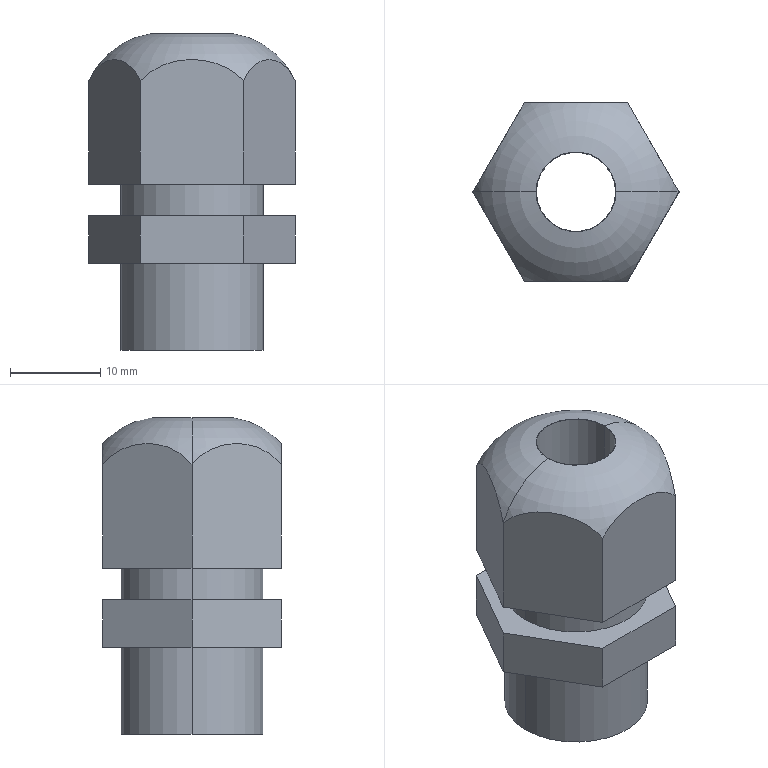Part | SolidWorks | features BaseBody 1 | 1 solid | 29 faces | box 22.88 x 19.815 x 35.2 mm | volume 6256 mm3 | plane 17 | cylinder 8 | cone 2 | torus 2 | commonest cylinder face diameters 15.84 x4 8.8 x2 12.32 x2
STEP:
#1=CARTESIAN_POINT('',(6.16,0.,21.12));
#2=VERTEX_POINT('',#1);
#3=CARTESIAN_POINT('',(-6.16,0.,21.12));
#4=VERTEX_POINT('',#3);
#5=CARTESIAN_POINT('',(0.,0.,21.12));
#6=DIRECTION('',(0.,0.,-1.));
#7=DIRECTION('',(-1.,0.,0.));
#8=AXIS2_PLACEMENT_3D('',#5,#6,#7);
#9=CIRCLE('',#8,6.16);
#10=EDGE_CURVE('',#2,#4,#9,.T.);
#11=ORIENTED_EDGE('',*,*,#10,.F.);
#12=CARTESIAN_POINT('',(6.16,0.,0.));
#13=VERTEX_POINT('',#12);
#14=CARTESIAN_POINT('',(6.16,0.,0.));
#15=DIRECTION('',(0.,0.,-1.));
#16=VECTOR('',#15,1000.);
#17=LINE('',#14,#16);
#18=EDGE_CURVE('',#2,#13,#17,.T.);
#19=ORIENTED_EDGE('',*,*,#18,.T.);
#20=CARTESIAN_POINT('',(-6.16,0.,0.));
#21=VERTEX_POINT('',#20);
#22=CARTESIAN_POINT('',(0.,0.,0.));
#23=DIRECTION('',(0.,0.,1.));
#24=DIRECTION('',(-1.,0.,0.));
#25=AXIS2_PLACEMENT_3D('',#22,#23,#24);
#26=CIRCLE('',#25,6.16);
#27=EDGE_CURVE('',#21,#13,#26,.T.);
#28=ORIENTED_EDGE('',*,*,#27,.F.);
#29=CARTESIAN_POINT('',(-6.16,0.,0.));
#30=DIRECTION('',(0.,0.,-1.));
#31=VECTOR('',#30,1000.);
#32=LINE('',#29,#31);
#33=EDGE_CURVE('',#4,#21,#32,.T.);
#34=ORIENTED_EDGE('',*,*,#33,.F.);
#35=EDGE_LOOP('',(#11,#19,#28,#34));
#36=FACE_OUTER_BOUND('',#35,.T.);
#37=CARTESIAN_POINT('',(0.,0.,0.));
#38=DIRECTION('',(0.,0.,-1.));
#39=DIRECTION('',(-1.,0.,0.));
#40=AXIS2_PLACEMENT_3D('',#37,#38,#39);
#41=CYLINDRICAL_SURFACE('',#40,6.16);
#42=ADVANCED_FACE('',(#36),#41,.F.);
#43=CARTESIAN_POINT('',(4.4,0.,22.754));
#44=VERTEX_POINT('',#43);
#45=CARTESIAN_POINT('',(-4.4,0.,22.754));
#46=VERTEX_POINT('',#45);
#47=CARTESIAN_POINT('',(0.,0.,22.754));
#48=DIRECTION('',(0.,0.,-1.));
#49=DIRECTION('',(1.,0.,0.));
#50=AXIS2_PLACEMENT_3D('',#47,#48,#49);
#51=CIRCLE('',#50,4.4);
#52=EDGE_CURVE('',#44,#46,#51,.T.);
#53=ORIENTED_EDGE('',*,*,#52,.F.);
#54=CARTESIAN_POINT('',(6.16,0.,21.12));
#55=DIRECTION('',(0.7329,0.,-0.6804));
#56=VECTOR('',#55,1000.);
#57=LINE('',#54,#56);
#58=EDGE_CURVE('',#44,#2,#57,.T.);
#59=ORIENTED_EDGE('',*,*,#58,.T.);
#60=ORIENTED_EDGE('',*,*,#10,.T.);
#61=CARTESIAN_POINT('',(-6.16,0.,21.12));
#62=DIRECTION('',(-0.7329,0.,-0.6804));
#63=VECTOR('',#62,1000.);
#64=LINE('',#61,#63);
#65=EDGE_CURVE('',#46,#4,#64,.T.);
#66=ORIENTED_EDGE('',*,*,#65,.F.);
#67=EDGE_LOOP('',(#53,#59,#60,#66));
#68=FACE_OUTER_BOUND('',#67,.T.);
#69=CARTESIAN_POINT('',(0.,0.,21.12));
#70=DIRECTION('',(0.,0.,-1.));
#71=DIRECTION('',(-1.,0.,0.));
#72=AXIS2_PLACEMENT_3D('',#69,#70,#71);
#73=CONICAL_SURFACE('',#72,6.16,0.8225);
#74=ADVANCED_FACE('',(#68),#73,.F.);
#75=CARTESIAN_POINT('',(-7.92,0.,9.68));
#76=VERTEX_POINT('',#75);
#77=CARTESIAN_POINT('',(7.92,0.,9.68));
#78=VERTEX_POINT('',#77);
#79=CARTESIAN_POINT('',(0.,0.,9.68));
#80=DIRECTION('',(0.,0.,-1.));
#81=DIRECTION('',(-1.,0.,0.));
#82=AXIS2_PLACEMENT_3D('',#79,#80,#81);
#83=CIRCLE('',#82,7.92);
#84=EDGE_CURVE('',#76,#78,#83,.T.);
#85=ORIENTED_EDGE('',*,*,#84,.T.);
#86=CARTESIAN_POINT('',(7.92,0.,0.));
#87=VERTEX_POINT('',#86);
#88=CARTESIAN_POINT('',(7.92,0.,0.));
#89=DIRECTION('',(0.,0.,-1.));
#90=VECTOR('',#89,1000.);
#91=LINE('',#88,#90);
#92=EDGE_CURVE('',#78,#87,#91,.T.);
#93=ORIENTED_EDGE('',*,*,#92,.T.);
#94=CARTESIAN_POINT('',(-7.92,0.,0.));
#95=VERTEX_POINT('',#94);
#96=CARTESIAN_POINT('',(0.,0.,0.));
#97=DIRECTION('',(0.,0.,1.));
#98=DIRECTION('',(-1.,0.,0.));
#99=AXIS2_PLACEMENT_3D('',#96,#97,#98);
#100=CIRCLE('',#99,7.92);
#101=EDGE_CURVE('',#87,#95,#100,.T.);
#102=ORIENTED_EDGE('',*,*,#101,.T.);
#103=CARTESIAN_POINT('',(-7.92,0.,0.));
#104=DIRECTION('',(0.,0.,-1.));
#105=VECTOR('',#104,1000.);
#106=LINE('',#103,#105);
#107=EDGE_CURVE('',#76,#95,#106,.T.);
#108=ORIENTED_EDGE('',*,*,#107,.F.);
#109=EDGE_LOOP('',(#85,#93,#102,#108));
#110=FACE_OUTER_BOUND('',#109,.T.);
#111=CARTESIAN_POINT('',(0.,0.,0.));
#112=DIRECTION('',(0.,0.,-1.));
#113=DIRECTION('',(-1.,0.,0.));
#114=AXIS2_PLACEMENT_3D('',#111,#112,#113);
#115=CYLINDRICAL_SURFACE('',#114,7.92);
#116=ADVANCED_FACE('',(#110),#115,.T.);
#117=CARTESIAN_POINT('',(4.4,0.,35.2));
#118=VERTEX_POINT('',#117);
#119=CARTESIAN_POINT('',(-4.4,0.,35.2));
#120=VERTEX_POINT('',#119);
#121=CARTESIAN_POINT('',(0.,0.,35.2));
#122=DIRECTION('',(0.,0.,-1.));
#123=DIRECTION('',(-1.,0.,0.));
#124=AXIS2_PLACEMENT_3D('',#121,#122,#123);
#125=CIRCLE('',#124,4.4);
#126=EDGE_CURVE('',#118,#120,#125,.T.);
#127=ORIENTED_EDGE('',*,*,#126,.F.);
#128=CARTESIAN_POINT('',(4.4,0.,0.));
#129=DIRECTION('',(0.,0.,-1.));
#130=VECTOR('',#129,1000.);
#131=LINE('',#128,#130);
#132=EDGE_CURVE('',#118,#44,#131,.T.);
#133=ORIENTED_EDGE('',*,*,#132,.T.);
#134=ORIENTED_EDGE('',*,*,#52,.T.);
#135=CARTESIAN_POINT('',(-4.4,0.,0.));
#136=DIRECTION('',(0.,0.,-1.));
#137=VECTOR('',#136,1000.);
#138=LINE('',#135,#137);
#139=EDGE_CURVE('',#120,#46,#138,.T.);
#140=ORIENTED_EDGE('',*,*,#139,.F.);
#141=EDGE_LOOP('',(#127,#133,#134,#140));
#142=FACE_OUTER_BOUND('',#141,.T.);
#143=CARTESIAN_POINT('',(0.,0.,0.));
#144=DIRECTION('',(0.,0.,-1.));
#145=DIRECTION('',(-1.,0.,0.));
#146=AXIS2_PLACEMENT_3D('',#143,#144,#145);
#147=CYLINDRICAL_SURFACE('',#146,4.4);
#148=ADVANCED_FACE('',(#142),#147,.F.);
#149=CARTESIAN_POINT('',(-5.72,9.907,29.944));
#150=VERTEX_POINT('',#149);
#151=CARTESIAN_POINT('',(-11.44,0.,29.944));
#152=VERTEX_POINT('',#151);
#153=CARTESIAN_POINT('',(-5.72,9.907,29.944));
#154=CARTESIAN_POINT('',(-5.898,9.599,30.347));
#155=CARTESIAN_POINT('',(-6.098,9.252,30.693));
#156=CARTESIAN_POINT('',(-6.536,8.494,31.288));
#157=CARTESIAN_POINT('',(-6.776,8.078,31.538));
#158=CARTESIAN_POINT('',(-7.27,7.223,31.929));
#159=CARTESIAN_POINT('',(-7.525,6.78,32.073));
#160=CARTESIAN_POINT('',(-8.052,5.868,32.266));
#161=CARTESIAN_POINT('',(-8.317,5.41,32.312));
#162=CARTESIAN_POINT('',(-8.714,4.722,32.312));
#163=CARTESIAN_POINT('',(-8.847,4.492,32.3));
#164=CARTESIAN_POINT('',(-9.113,4.031,32.252));
#165=CARTESIAN_POINT('',(-9.246,3.801,32.215));
#166=CARTESIAN_POINT('',(-9.637,3.123,32.071));
#167=CARTESIAN_POINT('',(-9.891,2.683,31.928));
#168=CARTESIAN_POINT('',(-10.383,1.832,31.539));
#169=CARTESIAN_POINT('',(-10.623,1.415,31.289));
#170=CARTESIAN_POINT('',(-11.061,0.6558,30.693));
#171=CARTESIAN_POINT('',(-11.262,0.3088,30.347));
#172=CARTESIAN_POINT('',(-11.44,0.,29.944));
#173=B_SPLINE_CURVE_WITH_KNOTS('',3,(#153,#154,#155,#156,#157,#158,#159,#160,#161,#162,#163,#164,#165,#166,#167,#168,#169,#170,#171,#172),.UNSPECIFIED.,.F.,.F.,(4,2,2,2,2,2,2,2,2,4),(0.,0.001585,0.00317,0.004755,0.00634,0.007132,0.007924,0.009509,0.01109,0.01268),.UNSPECIFIED.);
#174=EDGE_CURVE('',#150,#152,#173,.T.);
#175=ORIENTED_EDGE('',*,*,#174,.T.);
#176=CARTESIAN_POINT('',(-4.446,0.,35.2));
#177=VERTEX_POINT('',#176);
#178=CARTESIAN_POINT('',(-3.243,0.,26.318));
#179=DIRECTION('',(0.,1.,0.));
#180=DIRECTION('',(-1.,0.,0.));
#181=AXIS2_PLACEMENT_3D('',#178,#179,#180);
#182=CIRCLE('',#181,8.963);
#183=EDGE_CURVE('',#152,#177,#182,.T.);
#184=ORIENTED_EDGE('',*,*,#183,.T.);
#185=CARTESIAN_POINT('',(4.446,0.,35.2));
#186=VERTEX_POINT('',#185);
#187=CARTESIAN_POINT('',(0.,0.,35.2));
#188=DIRECTION('',(0.,0.,1.));
#189=DIRECTION('',(1.,0.,0.));
#190=AXIS2_PLACEMENT_3D('',#187,#188,#189);
#191=CIRCLE('',#190,4.446);
#192=EDGE_CURVE('',#186,#177,#191,.T.);
#193=ORIENTED_EDGE('',*,*,#192,.F.);
#194=CARTESIAN_POINT('',(11.44,0.,29.944));
#195=VERTEX_POINT('',#194);
#196=CARTESIAN_POINT('',(3.243,0.,26.318));
#197=DIRECTION('',(0.,-1.,0.));
#198=DIRECTION('',(0.,0.,-1.));
#199=AXIS2_PLACEMENT_3D('',#196,#197,#198);
#200=CIRCLE('',#199,8.963);
#201=EDGE_CURVE('',#195,#186,#200,.T.);
#202=ORIENTED_EDGE('',*,*,#201,.F.);
#203=CARTESIAN_POINT('',(5.72,9.907,29.944));
#204=VERTEX_POINT('',#203);
#205=CARTESIAN_POINT('',(11.44,0.,29.944));
#206=CARTESIAN_POINT('',(11.262,0.3085,30.347));
#207=CARTESIAN_POINT('',(11.062,0.6552,30.693));
#208=CARTESIAN_POINT('',(10.624,1.413,31.288));
#209=CARTESIAN_POINT('',(10.384,1.829,31.538));
#210=CARTESIAN_POINT('',(9.89,2.684,31.929));
#211=CARTESIAN_POINT('',(9.635,3.127,32.073));
#212=CARTESIAN_POINT('',(9.108,4.04,32.266));
#213=CARTESIAN_POINT('',(8.843,4.497,32.312));
#214=CARTESIAN_POINT('',(8.446,5.186,32.312));
#215=CARTESIAN_POINT('',(8.313,5.416,32.3));
#216=CARTESIAN_POINT('',(8.047,5.876,32.252));
#217=CARTESIAN_POINT('',(7.914,6.106,32.215));
#218=CARTESIAN_POINT('',(7.523,6.784,32.071));
#219=CARTESIAN_POINT('',(7.269,7.224,31.928));
#220=CARTESIAN_POINT('',(6.777,8.076,31.539));
#221=CARTESIAN_POINT('',(6.537,8.492,31.289));
#222=CARTESIAN_POINT('',(6.099,9.252,30.693));
#223=CARTESIAN_POINT('',(5.898,9.599,30.347));
#224=CARTESIAN_POINT('',(5.72,9.907,29.944));
#225=B_SPLINE_CURVE_WITH_KNOTS('',3,(#205,#206,#207,#208,#209,#210,#211,#212,#213,#214,#215,#216,#217,#218,#219,#220,#221,#222,#223,#224),.UNSPECIFIED.,.F.,.F.,(4,2,2,2,2,2,2,2,2,4),(0.,0.001585,0.00317,0.004755,0.00634,0.007132,0.007924,0.009509,0.01109,0.01268),.UNSPECIFIED.);
#226=EDGE_CURVE('',#195,#204,#225,.T.);
#227=ORIENTED_EDGE('',*,*,#226,.T.);
#228=CARTESIAN_POINT('',(5.72,9.907,29.944));
#229=CARTESIAN_POINT('',(5.364,9.907,30.347));
#230=CARTESIAN_POINT('',(4.963,9.907,30.693));
#231=CARTESIAN_POINT('',(4.088,9.907,31.288));
#232=CARTESIAN_POINT('',(3.608,9.907,31.538));
#233=CARTESIAN_POINT('',(2.621,9.907,31.929));
#234=CARTESIAN_POINT('',(2.109,9.907,32.073));
#235=CARTESIAN_POINT('',(1.056,9.907,32.266));
#236=CARTESIAN_POINT('',(0.527,9.907,32.312));
#237=CARTESIAN_POINT('',(-0.2681,9.907,32.312));
#238=CARTESIAN_POINT('',(-0.5335,9.907,32.3));
#239=CARTESIAN_POINT('',(-1.065,9.907,32.252));
#240=CARTESIAN_POINT('',(-1.331,9.907,32.215));
#241=CARTESIAN_POINT('',(-2.114,9.907,32.071));
#242=CARTESIAN_POINT('',(-2.621,9.907,31.928));
#243=CARTESIAN_POINT('',(-3.605,9.907,31.539));
#244=CARTESIAN_POINT('',(-4.086,9.907,31.289));
#245=CARTESIAN_POINT('',(-4.963,9.907,30.693));
#246=CARTESIAN_POINT('',(-5.363,9.907,30.347));
#247=CARTESIAN_POINT('',(-5.72,9.907,29.944));
#248=B_SPLINE_CURVE_WITH_KNOTS('',3,(#228,#229,#230,#231,#232,#233,#234,#235,#236,#237,#238,#239,#240,#241,#242,#243,#244,#245,#246,#247),.UNSPECIFIED.,.F.,.F.,(4,2,2,2,2,2,2,2,2,4),(0.,0.001585,0.00317,0.004755,0.00634,0.007132,0.007924,0.009509,0.01109,0.01268),.UNSPECIFIED.);
#249=EDGE_CURVE('',#204,#150,#248,.T.);
#250=ORIENTED_EDGE('',*,*,#249,.T.);
#251=EDGE_LOOP('',(#175,#184,#193,#202,#227,#250));
#252=FACE_OUTER_BOUND('',#251,.T.);
#253=CARTESIAN_POINT('',(0.,0.,26.318));
#254=DIRECTION('',(0.,0.,1.));
#255=DIRECTION('',(1.,0.,0.));
#256=AXIS2_PLACEMENT_3D('',#253,#254,#255);
#257=TOROIDAL_SURFACE('',#256,3.243,8.963);
#258=ADVANCED_FACE('',(#252),#257,.T.);
#259=CARTESIAN_POINT('',(-7.92,0.,18.48));
#260=VERTEX_POINT('',#259);
#261=CARTESIAN_POINT('',(7.92,0.,18.48));
#262=VERTEX_POINT('',#261);
#263=CARTESIAN_POINT('',(0.,0.,18.48));
#264=DIRECTION('',(0.,0.,-1.));
#265=DIRECTION('',(-1.,0.,0.));
#266=AXIS2_PLACEMENT_3D('',#263,#264,#265);
#267=CIRCLE('',#266,7.92);
#268=EDGE_CURVE('',#260,#262,#267,.T.);
#269=ORIENTED_EDGE('',*,*,#268,.T.);
#270=CARTESIAN_POINT('',(7.92,0.,14.96));
#271=VERTEX_POINT('',#270);
#272=CARTESIAN_POINT('',(7.92,0.,0.));
#273=DIRECTION('',(0.,0.,-1.));
#274=VECTOR('',#273,1000.);
#275=LINE('',#272,#274);
#276=EDGE_CURVE('',#262,#271,#275,.T.);
#277=ORIENTED_EDGE('',*,*,#276,.T.);
#278=CARTESIAN_POINT('',(-7.92,0.,14.96));
#279=VERTEX_POINT('',#278);
#280=CARTESIAN_POINT('',(0.,0.,14.96));
#281=DIRECTION('',(0.,0.,1.));
#282=DIRECTION('',(-1.,0.,0.));
#283=AXIS2_PLACEMENT_3D('',#280,#281,#282);
#284=CIRCLE('',#283,7.92);
#285=EDGE_CURVE('',#271,#279,#284,.T.);
#286=ORIENTED_EDGE('',*,*,#285,.T.);
#287=CARTESIAN_POINT('',(-7.92,0.,0.));
#288=DIRECTION('',(0.,0.,-1.));
#289=VECTOR('',#288,1000.);
#290=LINE('',#287,#289);
#291=EDGE_CURVE('',#260,#279,#290,.T.);
#292=ORIENTED_EDGE('',*,*,#291,.F.);
#293=EDGE_LOOP('',(#269,#277,#286,#292));
#294=FACE_OUTER_BOUND('',#293,.T.);
#295=CARTESIAN_POINT('',(0.,0.,0.));
#296=DIRECTION('',(0.,0.,-1.));
#297=DIRECTION('',(-1.,0.,0.));
#298=AXIS2_PLACEMENT_3D('',#295,#296,#297);
#299=CYLINDRICAL_SURFACE('',#298,7.92);
#300=ADVANCED_FACE('',(#294),#299,.T.);
#301=ORIENTED_EDGE('',*,*,#18,.F.);
#302=CARTESIAN_POINT('',(0.,0.,21.12));
#303=DIRECTION('',(0.,0.,-1.));
#304=DIRECTION('',(-1.,0.,0.));
#305=AXIS2_PLACEMENT_3D('',#302,#303,#304);
#306=CIRCLE('',#305,6.16);
#307=EDGE_CURVE('',#4,#2,#306,.T.);
#308=ORIENTED_EDGE('',*,*,#307,.F.);
#309=ORIENTED_EDGE('',*,*,#33,.T.);
#310=CARTESIAN_POINT('',(0.,0.,0.));
#311=DIRECTION('',(0.,0.,1.));
#312=DIRECTION('',(-1.,0.,0.));
#313=AXIS2_PLACEMENT_3D('',#310,#311,#312);
#314=CIRCLE('',#313,6.16);
#315=EDGE_CURVE('',#13,#21,#314,.T.);
#316=ORIENTED_EDGE('',*,*,#315,.F.);
#317=EDGE_LOOP('',(#301,#308,#309,#316));
#318=FACE_OUTER_BOUND('',#317,.T.);
#319=CARTESIAN_POINT('',(0.,0.,0.));
#320=DIRECTION('',(0.,0.,-1.));
#321=DIRECTION('',(-1.,0.,0.));
#322=AXIS2_PLACEMENT_3D('',#319,#320,#321);
#323=CYLINDRICAL_SURFACE('',#322,6.16);
#324=ADVANCED_FACE('',(#318),#323,.F.);
#325=ORIENTED_EDGE('',*,*,#27,.T.);
#326=ORIENTED_EDGE('',*,*,#315,.T.);
#327=EDGE_LOOP('',(#325,#326));
#328=FACE_BOUND('',#327,.T.);
#329=CARTESIAN_POINT('',(0.,0.,0.));
#330=DIRECTION('',(0.,0.,1.));
#331=DIRECTION('',(-1.,0.,0.));
#332=AXIS2_PLACEMENT_3D('',#329,#330,#331);
#333=CIRCLE('',#332,7.92);
#334=EDGE_CURVE('',#95,#87,#333,.T.);
#335=ORIENTED_EDGE('',*,*,#334,.F.);
#336=ORIENTED_EDGE('',*,*,#101,.F.);
#337=EDGE_LOOP('',(#335,#336));
#338=FACE_OUTER_BOUND('',#337,.T.);
#339=CARTESIAN_POINT('',(-11.44,-9.907,0.));
#340=DIRECTION('',(0.,0.,1.));
#341=DIRECTION('',(1.,0.,0.));
#342=AXIS2_PLACEMENT_3D('',#339,#340,#341);
#343=PLANE('',#342);
#344=ADVANCED_FACE('',(#328,#338),#343,.F.);
#345=ORIENTED_EDGE('',*,*,#58,.F.);
#346=CARTESIAN_POINT('',(0.,0.,22.754));
#347=DIRECTION('',(0.,0.,-1.));
#348=DIRECTION('',(1.,0.,0.));
#349=AXIS2_PLACEMENT_3D('',#346,#347,#348);
#350=CIRCLE('',#349,4.4);
#351=EDGE_CURVE('',#46,#44,#350,.T.);
#352=ORIENTED_EDGE('',*,*,#351,.F.);
#353=ORIENTED_EDGE('',*,*,#65,.T.);
#354=ORIENTED_EDGE('',*,*,#307,.T.);
#355=EDGE_LOOP('',(#345,#352,#353,#354));
#356=FACE_OUTER_BOUND('',#355,.T.);
#357=CARTESIAN_POINT('',(0.,0.,21.12));
#358=DIRECTION('',(0.,0.,-1.));
#359=DIRECTION('',(-1.,0.,0.));
#360=AXIS2_PLACEMENT_3D('',#357,#358,#359);
#361=CONICAL_SURFACE('',#360,6.16,0.8225);
#362=ADVANCED_FACE('',(#356),#361,.F.);
#363=ORIENTED_EDGE('',*,*,#92,.F.);
#364=CARTESIAN_POINT('',(0.,0.,9.68));
#365=DIRECTION('',(0.,0.,-1.));
#366=DIRECTION('',(-1.,0.,0.));
#367=AXIS2_PLACEMENT_3D('',#364,#365,#366);
#368=CIRCLE('',#367,7.92);
#369=EDGE_CURVE('',#78,#76,#368,.T.);
#370=ORIENTED_EDGE('',*,*,#369,.T.);
#371=ORIENTED_EDGE('',*,*,#107,.T.);
#372=ORIENTED_EDGE('',*,*,#334,.T.);
#373=EDGE_LOOP('',(#363,#370,#371,#372));
#374=FACE_OUTER_BOUND('',#373,.T.);
#375=CARTESIAN_POINT('',(0.,0.,0.));
#376=DIRECTION('',(0.,0.,-1.));
#377=DIRECTION('',(-1.,0.,0.));
#378=AXIS2_PLACEMENT_3D('',#375,#376,#377);
#379=CYLINDRICAL_SURFACE('',#378,7.92);
#380=ADVANCED_FACE('',(#374),#379,.T.);
#381=ORIENTED_EDGE('',*,*,#132,.F.);
#382=CARTESIAN_POINT('',(0.,0.,35.2));
#383=DIRECTION('',(0.,0.,-1.));
#384=DIRECTION('',(-1.,0.,0.));
#385=AXIS2_PLACEMENT_3D('',#382,#383,#384);
#386=CIRCLE('',#385,4.4);
#387=EDGE_CURVE('',#120,#118,#386,.T.);
#388=ORIENTED_EDGE('',*,*,#387,.F.);
#389=ORIENTED_EDGE('',*,*,#139,.T.);
#390=ORIENTED_EDGE('',*,*,#351,.T.);
#391=EDGE_LOOP('',(#381,#388,#389,#390));
#392=FACE_OUTER_BOUND('',#391,.T.);
#393=CARTESIAN_POINT('',(0.,0.,0.));
#394=DIRECTION('',(0.,0.,-1.));
#395=DIRECTION('',(-1.,0.,0.));
#396=AXIS2_PLACEMENT_3D('',#393,#394,#395);
#397=CYLINDRICAL_SURFACE('',#396,4.4);
#398=ADVANCED_FACE('',(#392),#397,.F.);
#399=CARTESIAN_POINT('',(-11.44,0.,9.68));
#400=VERTEX_POINT('',#399);
#401=CARTESIAN_POINT('',(-5.72,-9.907,9.68));
#402=VERTEX_POINT('',#401);
#403=CARTESIAN_POINT('',(-11.44,0.,9.68));
#404=DIRECTION('',(0.5,-0.866,0.));
#405=VECTOR('',#404,1000.);
#406=LINE('',#403,#405);
#407=EDGE_CURVE('',#400,#402,#406,.T.);
#408=ORIENTED_EDGE('',*,*,#407,.F.);
#409=CARTESIAN_POINT('',(-5.72,9.907,9.68));
#410=VERTEX_POINT('',#409);
#411=CARTESIAN_POINT('',(-5.72,9.907,9.68));
#412=DIRECTION('',(-0.5,-0.866,0.));
#413=VECTOR('',#412,1000.);
#414=LINE('',#411,#413);
#415=EDGE_CURVE('',#410,#400,#414,.T.);
#416=ORIENTED_EDGE('',*,*,#415,.F.);
#417=CARTESIAN_POINT('',(5.72,9.907,9.68));
#418=VERTEX_POINT('',#417);
#419=CARTESIAN_POINT('',(0.,9.907,9.68));
#420=DIRECTION('',(-1.,0.,0.));
#421=VECTOR('',#420,1000.);
#422=LINE('',#419,#421);
#423=EDGE_CURVE('',#418,#410,#422,.T.);
#424=ORIENTED_EDGE('',*,*,#423,.F.);
#425=CARTESIAN_POINT('',(11.44,0.,9.68));
#426=VERTEX_POINT('',#425);
#427=CARTESIAN_POINT('',(11.44,0.,9.68));
#428=DIRECTION('',(-0.5,0.866,0.));
#429=VECTOR('',#428,1000.);
#430=LINE('',#427,#429);
#431=EDGE_CURVE('',#426,#418,#430,.T.);
#432=ORIENTED_EDGE('',*,*,#431,.F.);
#433=CARTESIAN_POINT('',(5.72,-9.907,9.68));
#434=VERTEX_POINT('',#433);
#435=CARTESIAN_POINT('',(5.72,-9.907,9.68));
#436=DIRECTION('',(0.5,0.866,0.));
#437=VECTOR('',#436,1000.);
#438=LINE('',#435,#437);
#439=EDGE_CURVE('',#434,#426,#438,.T.);
#440=ORIENTED_EDGE('',*,*,#439,.F.);
#441=CARTESIAN_POINT('',(0.,-9.907,9.68));
#442=DIRECTION('',(1.,0.,0.));
#443=VECTOR('',#442,1000.);
#444=LINE('',#441,#443);
#445=EDGE_CURVE('',#402,#434,#444,.T.);
#446=ORIENTED_EDGE('',*,*,#445,.F.);
#447=EDGE_LOOP('',(#408,#416,#424,#432,#440,#446));
#448=FACE_OUTER_BOUND('',#447,.T.);
#449=ORIENTED_EDGE('',*,*,#84,.F.);
#450=ORIENTED_EDGE('',*,*,#369,.F.);
#451=EDGE_LOOP('',(#449,#450));
#452=FACE_BOUND('',#451,.T.);
#453=CARTESIAN_POINT('',(0.,-14.206,9.68));
#454=DIRECTION('',(0.,0.,1.));
#455=DIRECTION('',(1.,0.,0.));
#456=AXIS2_PLACEMENT_3D('',#453,#454,#455);
#457=PLANE('',#456);
#458=ADVANCED_FACE('',(#448,#452),#457,.F.);
#459=ORIENTED_EDGE('',*,*,#192,.T.);
#460=CARTESIAN_POINT('',(0.,0.,35.2));
#461=DIRECTION('',(0.,0.,1.));
#462=DIRECTION('',(1.,0.,0.));
#463=AXIS2_PLACEMENT_3D('',#460,#461,#462);
#464=CIRCLE('',#463,4.446);
#465=EDGE_CURVE('',#177,#186,#464,.T.);
#466=ORIENTED_EDGE('',*,*,#465,.T.);
#467=EDGE_LOOP('',(#459,#466));
#468=FACE_OUTER_BOUND('',#467,.T.);
#469=ORIENTED_EDGE('',*,*,#387,.T.);
#470=ORIENTED_EDGE('',*,*,#126,.T.);
#471=EDGE_LOOP('',(#469,#470));
#472=FACE_BOUND('',#471,.T.);
#473=CARTESIAN_POINT('',(-11.44,-9.907,35.2));
#474=DIRECTION('',(0.,0.,1.));
#475=DIRECTION('',(1.,0.,0.));
#476=AXIS2_PLACEMENT_3D('',#473,#474,#475);
#477=PLANE('',#476);
#478=ADVANCED_FACE('',(#468,#472),#477,.T.);
#479=ORIENTED_EDGE('',*,*,#445,.T.);
#480=CARTESIAN_POINT('',(5.72,-9.907,14.96));
#481=VERTEX_POINT('',#480);
#482=CARTESIAN_POINT('',(5.72,-9.907,35.2));
#483=DIRECTION('',(0.,0.,-1.));
#484=VECTOR('',#483,1000.);
#485=LINE('',#482,#484);
#486=EDGE_CURVE('',#481,#434,#485,.T.);
#487=ORIENTED_EDGE('',*,*,#486,.F.);
#488=CARTESIAN_POINT('',(-5.72,-9.907,14.96));
#489=VERTEX_POINT('',#488);
#490=CARTESIAN_POINT('',(-5.72,-9.907,14.96));
#491=DIRECTION('',(1.,0.,0.));
#492=VECTOR('',#491,1000.);
#493=LINE('',#490,#492);
#494=EDGE_CURVE('',#489,#481,#493,.T.);
#495=ORIENTED_EDGE('',*,*,#494,.F.);
#496=CARTESIAN_POINT('',(-5.72,-9.907,35.2));
#497=DIRECTION('',(0.,0.,1.));
#498=VECTOR('',#497,1000.);
#499=LINE('',#496,#498);
#500=EDGE_CURVE('',#402,#489,#499,.T.);
#501=ORIENTED_EDGE('',*,*,#500,.F.);
#502=EDGE_LOOP('',(#479,#487,#495,#501));
#503=FACE_OUTER_BOUND('',#502,.T.);
#504=CARTESIAN_POINT('',(-5.72,-9.907,35.2));
#505=DIRECTION('',(0.,1.,0.));
#506=DIRECTION('',(-1.,0.,0.));
#507=AXIS2_PLACEMENT_3D('',#504,#505,#506);
#508=PLANE('',#507);
#509=ADVANCED_FACE('',(#503),#508,.F.);
#510=ORIENTED_EDGE('',*,*,#407,.T.);
#511=ORIENTED_EDGE('',*,*,#500,.T.);
#512=CARTESIAN_POINT('',(-11.44,0.,14.96));
#513=VERTEX_POINT('',#512);
#514=CARTESIAN_POINT('',(-11.44,0.,14.96));
#515=DIRECTION('',(0.5,-0.866,0.));
#516=VECTOR('',#515,1000.);
#517=LINE('',#514,#516);
#518=EDGE_CURVE('',#513,#489,#517,.T.);
#519=ORIENTED_EDGE('',*,*,#518,.F.);
#520=CARTESIAN_POINT('',(-11.44,0.,35.2));
#521=DIRECTION('',(0.,0.,1.));
#522=VECTOR('',#521,1000.);
#523=LINE('',#520,#522);
#524=EDGE_CURVE('',#400,#513,#523,.T.);
#525=ORIENTED_EDGE('',*,*,#524,.F.);
#526=EDGE_LOOP('',(#510,#511,#519,#525));
#527=FACE_OUTER_BOUND('',#526,.T.);
#528=CARTESIAN_POINT('',(-11.44,0.,35.2));
#529=DIRECTION('',(0.866,0.5,0.));
#530=DIRECTION('',(-0.5,0.866,0.));
#531=AXIS2_PLACEMENT_3D('',#528,#529,#530);
#532=PLANE('',#531);
#533=ADVANCED_FACE('',(#527),#532,.F.);
#534=ORIENTED_EDGE('',*,*,#415,.T.);
#535=ORIENTED_EDGE('',*,*,#524,.T.);
#536=CARTESIAN_POINT('',(-5.72,9.907,14.96));
#537=VERTEX_POINT('',#536);
#538=CARTESIAN_POINT('',(-5.72,9.907,14.96));
#539=DIRECTION('',(-0.5,-0.866,0.));
#540=VECTOR('',#539,1000.);
#541=LINE('',#538,#540);
#542=EDGE_CURVE('',#537,#513,#541,.T.);
#543=ORIENTED_EDGE('',*,*,#542,.F.);
#544=CARTESIAN_POINT('',(-5.72,9.907,35.2));
#545=DIRECTION('',(0.,0.,1.));
#546=VECTOR('',#545,1000.);
#547=LINE('',#544,#546);
#548=EDGE_CURVE('',#410,#537,#547,.T.);
#549=ORIENTED_EDGE('',*,*,#548,.F.);
#550=EDGE_LOOP('',(#534,#535,#543,#549));
#551=FACE_OUTER_BOUND('',#550,.T.);
#552=CARTESIAN_POINT('',(-5.72,9.907,35.2));
#553=DIRECTION('',(0.866,-0.5,0.));
#554=DIRECTION('',(0.5,0.866,0.));
#555=AXIS2_PLACEMENT_3D('',#552,#553,#554);
#556=PLANE('',#555);
#557=ADVANCED_FACE('',(#551),#556,.F.);
#558=ORIENTED_EDGE('',*,*,#423,.T.);
#559=ORIENTED_EDGE('',*,*,#548,.T.);
#560=CARTESIAN_POINT('',(5.72,9.907,14.96));
#561=VERTEX_POINT('',#560);
#562=CARTESIAN_POINT('',(5.72,9.907,14.96));
#563=DIRECTION('',(-1.,0.,0.));
#564=VECTOR('',#563,1000.);
#565=LINE('',#562,#564);
#566=EDGE_CURVE('',#561,#537,#565,.T.);
#567=ORIENTED_EDGE('',*,*,#566,.F.);
#568=CARTESIAN_POINT('',(5.72,9.907,35.2));
#569=DIRECTION('',(0.,0.,1.));
#570=VECTOR('',#569,1000.);
#571=LINE('',#568,#570);
#572=EDGE_CURVE('',#418,#561,#571,.T.);
#573=ORIENTED_EDGE('',*,*,#572,.F.);
#574=EDGE_LOOP('',(#558,#559,#567,#573));
#575=FACE_OUTER_BOUND('',#574,.T.);
#576=CARTESIAN_POINT('',(5.72,9.907,35.2));
#577=DIRECTION('',(0.,-1.,0.));
#578=DIRECTION('',(0.,0.,-1.));
#579=AXIS2_PLACEMENT_3D('',#576,#577,#578);
#580=PLANE('',#579);
#581=ADVANCED_FACE('',(#575),#580,.F.);
#582=ORIENTED_EDGE('',*,*,#431,.T.);
#583=ORIENTED_EDGE('',*,*,#572,.T.);
#584=CARTESIAN_POINT('',(11.44,0.,14.96));
#585=VERTEX_POINT('',#584);
#586=CARTESIAN_POINT('',(11.44,0.,14.96));
#587=DIRECTION('',(-0.5,0.866,0.));
#588=VECTOR('',#587,1000.);
#589=LINE('',#586,#588);
#590=EDGE_CURVE('',#585,#561,#589,.T.);
#591=ORIENTED_EDGE('',*,*,#590,.F.);
#592=CARTESIAN_POINT('',(11.44,0.,35.2));
#593=DIRECTION('',(0.,0.,1.));
#594=VECTOR('',#593,1000.);
#595=LINE('',#592,#594);
#596=EDGE_CURVE('',#426,#585,#595,.T.);
#597=ORIENTED_EDGE('',*,*,#596,.F.);
#598=EDGE_LOOP('',(#582,#583,#591,#597));
#599=FACE_OUTER_BOUND('',#598,.T.);
#600=CARTESIAN_POINT('',(11.44,0.,35.2));
#601=DIRECTION('',(-0.866,-0.5,0.));
#602=DIRECTION('',(0.5,-0.866,0.));
#603=AXIS2_PLACEMENT_3D('',#600,#601,#602);
#604=PLANE('',#603);
#605=ADVANCED_FACE('',(#599),#604,.F.);
#606=ORIENTED_EDGE('',*,*,#439,.T.);
#607=ORIENTED_EDGE('',*,*,#596,.T.);
#608=CARTESIAN_POINT('',(5.72,-9.907,14.96));
#609=DIRECTION('',(0.5,0.866,0.));
#610=VECTOR('',#609,1000.);
#611=LINE('',#608,#610);
#612=EDGE_CURVE('',#481,#585,#611,.T.);
#613=ORIENTED_EDGE('',*,*,#612,.F.);
#614=ORIENTED_EDGE('',*,*,#486,.T.);
#615=EDGE_LOOP('',(#606,#607,#613,#614));
#616=FACE_OUTER_BOUND('',#615,.T.);
#617=CARTESIAN_POINT('',(5.72,-9.907,35.2));
#618=DIRECTION('',(-0.866,0.5,0.));
#619=DIRECTION('',(-0.5,-0.866,0.));
#620=AXIS2_PLACEMENT_3D('',#617,#618,#619);
#621=PLANE('',#620);
#622=ADVANCED_FACE('',(#616),#621,.F.);
#623=ORIENTED_EDGE('',*,*,#183,.F.);
#624=CARTESIAN_POINT('',(-5.72,-9.907,29.944));
#625=VERTEX_POINT('',#624);
#626=CARTESIAN_POINT('',(-11.44,0.,29.944));
#627=CARTESIAN_POINT('',(-11.262,-0.3085,30.347));
#628=CARTESIAN_POINT('',(-11.062,-0.6552,30.693));
#629=CARTESIAN_POINT('',(-10.624,-1.413,31.288));
#630=CARTESIAN_POINT('',(-10.384,-1.829,31.538));
#631=CARTESIAN_POINT('',(-9.89,-2.684,31.929));
#632=CARTESIAN_POINT('',(-9.635,-3.127,32.073));
#633=CARTESIAN_POINT('',(-9.108,-4.04,32.266));
#634=CARTESIAN_POINT('',(-8.843,-4.497,32.312));
#635=CARTESIAN_POINT('',(-8.446,-5.186,32.312));
#636=CARTESIAN_POINT('',(-8.313,-5.416,32.3));
#637=CARTESIAN_POINT('',(-8.047,-5.876,32.252));
#638=CARTESIAN_POINT('',(-7.914,-6.106,32.215));
#639=CARTESIAN_POINT('',(-7.523,-6.784,32.071));
#640=CARTESIAN_POINT('',(-7.269,-7.224,31.928));
#641=CARTESIAN_POINT('',(-6.777,-8.076,31.539));
#642=CARTESIAN_POINT('',(-6.537,-8.492,31.289));
#643=CARTESIAN_POINT('',(-6.099,-9.252,30.693));
#644=CARTESIAN_POINT('',(-5.898,-9.599,30.347));
#645=CARTESIAN_POINT('',(-5.72,-9.907,29.944));
#646=B_SPLINE_CURVE_WITH_KNOTS('',3,(#626,#627,#628,#629,#630,#631,#632,#633,#634,#635,#636,#637,#638,#639,#640,#641,#642,#643,#644,#645),.UNSPECIFIED.,.F.,.F.,(4,2,2,2,2,2,2,2,2,4),(0.,0.001585,0.00317,0.004755,0.00634,0.007132,0.007924,0.009509,0.01109,0.01268),.UNSPECIFIED.);
#647=EDGE_CURVE('',#152,#625,#646,.T.);
#648=ORIENTED_EDGE('',*,*,#647,.T.);
#649=CARTESIAN_POINT('',(5.72,-9.907,29.944));
#650=VERTEX_POINT('',#649);
#651=CARTESIAN_POINT('',(-5.72,-9.907,29.944));
#652=CARTESIAN_POINT('',(-5.364,-9.907,30.347));
#653=CARTESIAN_POINT('',(-4.963,-9.907,30.693));
#654=CARTESIAN_POINT('',(-4.088,-9.907,31.288));
#655=CARTESIAN_POINT('',(-3.608,-9.907,31.538));
#656=CARTESIAN_POINT('',(-2.621,-9.907,31.929));
#657=CARTESIAN_POINT('',(-2.109,-9.907,32.073));
#658=CARTESIAN_POINT('',(-1.056,-9.907,32.266));
#659=CARTESIAN_POINT('',(-0.527,-9.907,32.312));
#660=CARTESIAN_POINT('',(0.2681,-9.907,32.312));
#661=CARTESIAN_POINT('',(0.5335,-9.907,32.3));
#662=CARTESIAN_POINT('',(1.065,-9.907,32.252));
#663=CARTESIAN_POINT('',(1.331,-9.907,32.215));
#664=CARTESIAN_POINT('',(2.114,-9.907,32.071));
#665=CARTESIAN_POINT('',(2.621,-9.907,31.928));
#666=CARTESIAN_POINT('',(3.605,-9.907,31.539));
#667=CARTESIAN_POINT('',(4.086,-9.907,31.289));
#668=CARTESIAN_POINT('',(4.963,-9.907,30.693));
#669=CARTESIAN_POINT('',(5.363,-9.907,30.347));
#670=CARTESIAN_POINT('',(5.72,-9.907,29.944));
#671=B_SPLINE_CURVE_WITH_KNOTS('',3,(#651,#652,#653,#654,#655,#656,#657,#658,#659,#660,#661,#662,#663,#664,#665,#666,#667,#668,#669,#670),.UNSPECIFIED.,.F.,.F.,(4,2,2,2,2,2,2,2,2,4),(0.,0.001585,0.00317,0.004755,0.00634,0.007132,0.007924,0.009509,0.01109,0.01268),.UNSPECIFIED.);
#672=EDGE_CURVE('',#625,#650,#671,.T.);
#673=ORIENTED_EDGE('',*,*,#672,.T.);
#674=CARTESIAN_POINT('',(5.72,-9.907,29.944));
#675=CARTESIAN_POINT('',(5.898,-9.599,30.347));
#676=CARTESIAN_POINT('',(6.098,-9.252,30.693));
#677=CARTESIAN_POINT('',(6.536,-8.494,31.288));
#678=CARTESIAN_POINT('',(6.776,-8.078,31.538));
#679=CARTESIAN_POINT('',(7.27,-7.223,31.929));
#680=CARTESIAN_POINT('',(7.525,-6.78,32.073));
#681=CARTESIAN_POINT('',(8.052,-5.868,32.266));
#682=CARTESIAN_POINT('',(8.317,-5.41,32.312));
#683=CARTESIAN_POINT('',(8.714,-4.722,32.312));
#684=CARTESIAN_POINT('',(8.847,-4.492,32.3));
#685=CARTESIAN_POINT('',(9.113,-4.031,32.252));
#686=CARTESIAN_POINT('',(9.246,-3.801,32.215));
#687=CARTESIAN_POINT('',(9.637,-3.123,32.071));
#688=CARTESIAN_POINT('',(9.891,-2.683,31.928));
#689=CARTESIAN_POINT('',(10.383,-1.832,31.539));
#690=CARTESIAN_POINT('',(10.623,-1.415,31.289));
#691=CARTESIAN_POINT('',(11.061,-0.6558,30.693));
#692=CARTESIAN_POINT('',(11.262,-0.3088,30.347));
#693=CARTESIAN_POINT('',(11.44,0.,29.944));
#694=B_SPLINE_CURVE_WITH_KNOTS('',3,(#674,#675,#676,#677,#678,#679,#680,#681,#682,#683,#684,#685,#686,#687,#688,#689,#690,#691,#692,#693),.UNSPECIFIED.,.F.,.F.,(4,2,2,2,2,2,2,2,2,4),(0.,0.001585,0.00317,0.004755,0.00634,0.007132,0.007924,0.009509,0.01109,0.01268),.UNSPECIFIED.);
#695=EDGE_CURVE('',#650,#195,#694,.T.);
#696=ORIENTED_EDGE('',*,*,#695,.T.);
#697=ORIENTED_EDGE('',*,*,#201,.T.);
#698=ORIENTED_EDGE('',*,*,#465,.F.);
#699=EDGE_LOOP('',(#623,#648,#673,#696,#697,#698));
#700=FACE_OUTER_BOUND('',#699,.T.);
#701=CARTESIAN_POINT('',(0.,0.,26.318));
#702=DIRECTION('',(0.,0.,1.));
#703=DIRECTION('',(1.,0.,0.));
#704=AXIS2_PLACEMENT_3D('',#701,#702,#703);
#705=TOROIDAL_SURFACE('',#704,3.243,8.963);
#706=ADVANCED_FACE('',(#700),#705,.T.);
#707=ORIENTED_EDGE('',*,*,#566,.T.);
#708=ORIENTED_EDGE('',*,*,#542,.T.);
#709=ORIENTED_EDGE('',*,*,#518,.T.);
#710=ORIENTED_EDGE('',*,*,#494,.T.);
#711=ORIENTED_EDGE('',*,*,#612,.T.);
#712=ORIENTED_EDGE('',*,*,#590,.T.);
#713=EDGE_LOOP('',(#707,#708,#709,#710,#711,#712));
#714=FACE_OUTER_BOUND('',#713,.T.);
#715=CARTESIAN_POINT('',(0.,0.,14.96));
#716=DIRECTION('',(0.,0.,1.));
#717=DIRECTION('',(-1.,0.,0.));
#718=AXIS2_PLACEMENT_3D('',#715,#716,#717);
#719=CIRCLE('',#718,7.92);
#720=EDGE_CURVE('',#279,#271,#719,.T.);
#721=ORIENTED_EDGE('',*,*,#720,.F.);
#722=ORIENTED_EDGE('',*,*,#285,.F.);
#723=EDGE_LOOP('',(#721,#722));
#724=FACE_BOUND('',#723,.T.);
#725=CARTESIAN_POINT('',(0.,-7.92,14.96));
#726=DIRECTION('',(0.,0.,-1.));
#727=DIRECTION('',(-1.,0.,0.));
#728=AXIS2_PLACEMENT_3D('',#725,#726,#727);
#729=PLANE('',#728);
#730=ADVANCED_FACE('',(#714,#724),#729,.F.);
#731=ORIENTED_EDGE('',*,*,#672,.F.);
#732=CARTESIAN_POINT('',(-5.72,-9.907,18.48));
#733=VERTEX_POINT('',#732);
#734=CARTESIAN_POINT('',(-5.72,-9.907,35.2));
#735=DIRECTION('',(0.,0.,1.));
#736=VECTOR('',#735,1000.);
#737=LINE('',#734,#736);
#738=EDGE_CURVE('',#733,#625,#737,.T.);
#739=ORIENTED_EDGE('',*,*,#738,.F.);
#740=CARTESIAN_POINT('',(5.72,-9.907,18.48));
#741=VERTEX_POINT('',#740);
#742=CARTESIAN_POINT('',(-5.72,-9.907,18.48));
#743=DIRECTION('',(-1.,0.,0.));
#744=VECTOR('',#743,1000.);
#745=LINE('',#742,#744);
#746=EDGE_CURVE('',#741,#733,#745,.T.);
#747=ORIENTED_EDGE('',*,*,#746,.F.);
#748=CARTESIAN_POINT('',(5.72,-9.907,35.2));
#749=DIRECTION('',(0.,0.,-1.));
#750=VECTOR('',#749,1000.);
#751=LINE('',#748,#750);
#752=EDGE_CURVE('',#650,#741,#751,.T.);
#753=ORIENTED_EDGE('',*,*,#752,.F.);
#754=EDGE_LOOP('',(#731,#739,#747,#753));
#755=FACE_OUTER_BOUND('',#754,.T.);
#756=CARTESIAN_POINT('',(-5.72,-9.907,35.2));
#757=DIRECTION('',(0.,1.,0.));
#758=DIRECTION('',(-1.,0.,0.));
#759=AXIS2_PLACEMENT_3D('',#756,#757,#758);
#760=PLANE('',#759);
#761=ADVANCED_FACE('',(#755),#760,.F.);
#762=ORIENTED_EDGE('',*,*,#647,.F.);
#763=CARTESIAN_POINT('',(-11.44,0.,18.48));
#764=VERTEX_POINT('',#763);
#765=CARTESIAN_POINT('',(-11.44,0.,35.2));
#766=DIRECTION('',(0.,0.,1.));
#767=VECTOR('',#766,1000.);
#768=LINE('',#765,#767);
#769=EDGE_CURVE('',#764,#152,#768,.T.);
#770=ORIENTED_EDGE('',*,*,#769,.F.);
#771=CARTESIAN_POINT('',(-11.44,0.,18.48));
#772=DIRECTION('',(-0.5,0.866,0.));
#773=VECTOR('',#772,1000.);
#774=LINE('',#771,#773);
#775=EDGE_CURVE('',#733,#764,#774,.T.);
#776=ORIENTED_EDGE('',*,*,#775,.F.);
#777=ORIENTED_EDGE('',*,*,#738,.T.);
#778=EDGE_LOOP('',(#762,#770,#776,#777));
#779=FACE_OUTER_BOUND('',#778,.T.);
#780=CARTESIAN_POINT('',(-11.44,0.,35.2));
#781=DIRECTION('',(0.866,0.5,0.));
#782=DIRECTION('',(-0.5,0.866,0.));
#783=AXIS2_PLACEMENT_3D('',#780,#781,#782);
#784=PLANE('',#783);
#785=ADVANCED_FACE('',(#779),#784,.F.);
#786=ORIENTED_EDGE('',*,*,#174,.F.);
#787=CARTESIAN_POINT('',(-5.72,9.907,18.48));
#788=VERTEX_POINT('',#787);
#789=CARTESIAN_POINT('',(-5.72,9.907,35.2));
#790=DIRECTION('',(0.,0.,1.));
#791=VECTOR('',#790,1000.);
#792=LINE('',#789,#791);
#793=EDGE_CURVE('',#788,#150,#792,.T.);
#794=ORIENTED_EDGE('',*,*,#793,.F.);
#795=CARTESIAN_POINT('',(-5.72,9.907,18.48));
#796=DIRECTION('',(0.5,0.866,0.));
#797=VECTOR('',#796,1000.);
#798=LINE('',#795,#797);
#799=EDGE_CURVE('',#764,#788,#798,.T.);
#800=ORIENTED_EDGE('',*,*,#799,.F.);
#801=ORIENTED_EDGE('',*,*,#769,.T.);
#802=EDGE_LOOP('',(#786,#794,#800,#801));
#803=FACE_OUTER_BOUND('',#802,.T.);
#804=CARTESIAN_POINT('',(-5.72,9.907,35.2));
#805=DIRECTION('',(0.866,-0.5,0.));
#806=DIRECTION('',(0.5,0.866,0.));
#807=AXIS2_PLACEMENT_3D('',#804,#805,#806);
#808=PLANE('',#807);
#809=ADVANCED_FACE('',(#803),#808,.F.);
#810=ORIENTED_EDGE('',*,*,#249,.F.);
#811=CARTESIAN_POINT('',(5.72,9.907,18.48));
#812=VERTEX_POINT('',#811);
#813=CARTESIAN_POINT('',(5.72,9.907,35.2));
#814=DIRECTION('',(0.,0.,1.));
#815=VECTOR('',#814,1000.);
#816=LINE('',#813,#815);
#817=EDGE_CURVE('',#812,#204,#816,.T.);
#818=ORIENTED_EDGE('',*,*,#817,.F.);
#819=CARTESIAN_POINT('',(5.72,9.907,18.48));
#820=DIRECTION('',(1.,0.,0.));
#821=VECTOR('',#820,1000.);
#822=LINE('',#819,#821);
#823=EDGE_CURVE('',#788,#812,#822,.T.);
#824=ORIENTED_EDGE('',*,*,#823,.F.);
#825=ORIENTED_EDGE('',*,*,#793,.T.);
#826=EDGE_LOOP('',(#810,#818,#824,#825));
#827=FACE_OUTER_BOUND('',#826,.T.);
#828=CARTESIAN_POINT('',(5.72,9.907,35.2));
#829=DIRECTION('',(0.,-1.,0.));
#830=DIRECTION('',(0.,0.,-1.));
#831=AXIS2_PLACEMENT_3D('',#828,#829,#830);
#832=PLANE('',#831);
#833=ADVANCED_FACE('',(#827),#832,.F.);
#834=ORIENTED_EDGE('',*,*,#226,.F.);
#835=CARTESIAN_POINT('',(11.44,0.,18.48));
#836=VERTEX_POINT('',#835);
#837=CARTESIAN_POINT('',(11.44,0.,35.2));
#838=DIRECTION('',(0.,0.,1.));
#839=VECTOR('',#838,1000.);
#840=LINE('',#837,#839);
#841=EDGE_CURVE('',#836,#195,#840,.T.);
#842=ORIENTED_EDGE('',*,*,#841,.F.);
#843=CARTESIAN_POINT('',(11.44,0.,18.48));
#844=DIRECTION('',(0.5,-0.866,0.));
#845=VECTOR('',#844,1000.);
#846=LINE('',#843,#845);
#847=EDGE_CURVE('',#812,#836,#846,.T.);
#848=ORIENTED_EDGE('',*,*,#847,.F.);
#849=ORIENTED_EDGE('',*,*,#817,.T.);
#850=EDGE_LOOP('',(#834,#842,#848,#849));
#851=FACE_OUTER_BOUND('',#850,.T.);
#852=CARTESIAN_POINT('',(11.44,0.,35.2));
#853=DIRECTION('',(-0.866,-0.5,0.));
#854=DIRECTION('',(0.5,-0.866,0.));
#855=AXIS2_PLACEMENT_3D('',#852,#853,#854);
#856=PLANE('',#855);
#857=ADVANCED_FACE('',(#851),#856,.F.);
#858=ORIENTED_EDGE('',*,*,#695,.F.);
#859=ORIENTED_EDGE('',*,*,#752,.T.);
#860=CARTESIAN_POINT('',(5.72,-9.907,18.48));
#861=DIRECTION('',(-0.5,-0.866,0.));
#862=VECTOR('',#861,1000.);
#863=LINE('',#860,#862);
#864=EDGE_CURVE('',#836,#741,#863,.T.);
#865=ORIENTED_EDGE('',*,*,#864,.F.);
#866=ORIENTED_EDGE('',*,*,#841,.T.);
#867=EDGE_LOOP('',(#858,#859,#865,#866));
#868=FACE_OUTER_BOUND('',#867,.T.);
#869=CARTESIAN_POINT('',(5.72,-9.907,35.2));
#870=DIRECTION('',(-0.866,0.5,0.));
#871=DIRECTION('',(-0.5,-0.866,0.));
#872=AXIS2_PLACEMENT_3D('',#869,#870,#871);
#873=PLANE('',#872);
#874=ADVANCED_FACE('',(#868),#873,.F.);
#875=ORIENTED_EDGE('',*,*,#276,.F.);
#876=CARTESIAN_POINT('',(0.,0.,18.48));
#877=DIRECTION('',(0.,0.,-1.));
#878=DIRECTION('',(-1.,0.,0.));
#879=AXIS2_PLACEMENT_3D('',#876,#877,#878);
#880=CIRCLE('',#879,7.92);
#881=EDGE_CURVE('',#262,#260,#880,.T.);
#882=ORIENTED_EDGE('',*,*,#881,.T.);
#883=ORIENTED_EDGE('',*,*,#291,.T.);
#884=ORIENTED_EDGE('',*,*,#720,.T.);
#885=EDGE_LOOP('',(#875,#882,#883,#884));
#886=FACE_OUTER_BOUND('',#885,.T.);
#887=CARTESIAN_POINT('',(0.,0.,0.));
#888=DIRECTION('',(0.,0.,-1.));
#889=DIRECTION('',(-1.,0.,0.));
#890=AXIS2_PLACEMENT_3D('',#887,#888,#889);
#891=CYLINDRICAL_SURFACE('',#890,7.92);
#892=ADVANCED_FACE('',(#886),#891,.T.);
#893=ORIENTED_EDGE('',*,*,#775,.T.);
#894=ORIENTED_EDGE('',*,*,#799,.T.);
#895=ORIENTED_EDGE('',*,*,#823,.T.);
#896=ORIENTED_EDGE('',*,*,#847,.T.);
#897=ORIENTED_EDGE('',*,*,#864,.T.);
#898=ORIENTED_EDGE('',*,*,#746,.T.);
#899=EDGE_LOOP('',(#893,#894,#895,#896,#897,#898));
#900=FACE_OUTER_BOUND('',#899,.T.);
#901=ORIENTED_EDGE('',*,*,#268,.F.);
#902=ORIENTED_EDGE('',*,*,#881,.F.);
#903=EDGE_LOOP('',(#901,#902));
#904=FACE_BOUND('',#903,.T.);
#905=CARTESIAN_POINT('',(0.,-11.586,18.48));
#906=DIRECTION('',(0.,0.,1.));
#907=DIRECTION('',(1.,0.,0.));
#908=AXIS2_PLACEMENT_3D('',#905,#906,#907);
#909=PLANE('',#908);
#910=ADVANCED_FACE('',(#900,#904),#909,.F.);
#911=CLOSED_SHELL('',(#42,#74,#116,#148,#258,#300,#324,#344,#362,#380,#398,#458,#478,#509,#533,#557,#581,#605,#622,#706,#730,#761,#785,#809,#833,#857,#874,#892,#910));
#912=MANIFOLD_SOLID_BREP('',#911);
#913=CARTESIAN_POINT('',(0.,0.,0.));
#914=DIRECTION('',(0.,0.,1.));
#915=DIRECTION('',(1.,0.,0.));
#916=AXIS2_PLACEMENT_3D('',#913,#914,#915);
#917=(LENGTH_UNIT()NAMED_UNIT(*)SI_UNIT(.MILLI.,.METRE.));
#918=UNCERTAINTY_MEASURE_WITH_UNIT(LENGTH_MEASURE(0.00001),#917,'','');
#919=(NAMED_UNIT(*)PLANE_ANGLE_UNIT()SI_UNIT($,.RADIAN.));
#920=(NAMED_UNIT(*)SI_UNIT($,.STERADIAN.)SOLID_ANGLE_UNIT());
#921=(GEOMETRIC_REPRESENTATION_CONTEXT(3)GLOBAL_UNCERTAINTY_ASSIGNED_CONTEXT((#918))GLOBAL_UNIT_ASSIGNED_CONTEXT((#917,#919,#920))REPRESENTATION_CONTEXT('',''));
#922=ADVANCED_BREP_SHAPE_REPRESENTATION('',(#912,#916),#921);